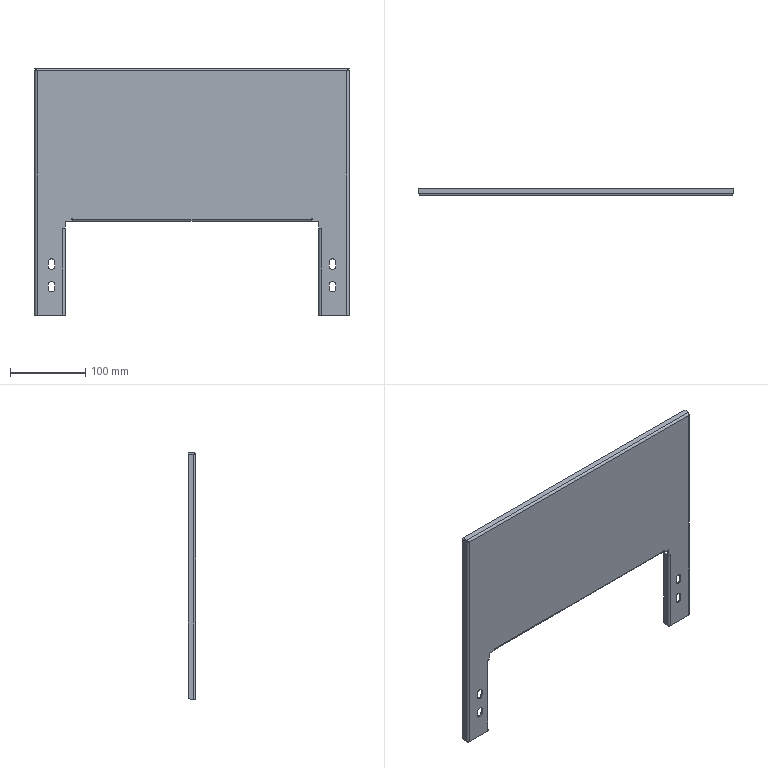Part | 1 solid | 100 faces | box 418 x 10 x 328 mm | volume 212187 mm3 | plane 67 | cylinder 29 | spline 4 | commonest cylinder face diameters 9 x12 1.48 x6 5.48 x6 8 x4 30 x1